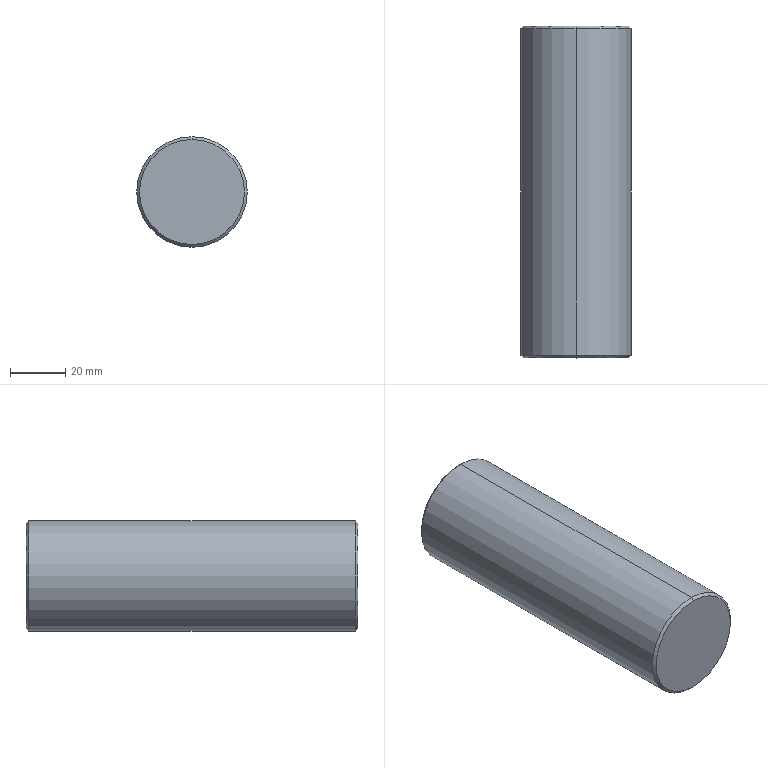Part | SolidWorks | 1 solid | 8 faces | box 40 x 120 x 40 mm | volume 150673 mm3 | cone 4 | cylinder 2 | plane 2 | commonest cylinder face diameters 40 x2
STEP:
#1=CARTESIAN_POINT('',(0.,0.,-19.));
#2=VERTEX_POINT('',#1);
#3=CARTESIAN_POINT('',(0.,0.,19.));
#4=VERTEX_POINT('',#3);
#5=CARTESIAN_POINT('',(0.,0.,0.));
#6=DIRECTION('',(0.,-1.,0.));
#7=DIRECTION('',(0.,0.,-1.));
#8=AXIS2_PLACEMENT_3D('',#5,#6,#7);
#9=CIRCLE('',#8,19.);
#10=EDGE_CURVE('',#2,#4,#9,.T.);
#11=ORIENTED_EDGE('',*,*,#10,.F.);
#12=CARTESIAN_POINT('',(0.,1.,-20.));
#13=VERTEX_POINT('',#12);
#14=CARTESIAN_POINT('',(0.,0.,-19.));
#15=DIRECTION('',(0.,0.7071,-0.7071));
#16=VECTOR('',#15,1000.);
#17=LINE('',#14,#16);
#18=EDGE_CURVE('',#2,#13,#17,.T.);
#19=ORIENTED_EDGE('',*,*,#18,.T.);
#20=CARTESIAN_POINT('',(0.,1.,20.));
#21=VERTEX_POINT('',#20);
#22=CARTESIAN_POINT('',(0.,1.,0.));
#23=DIRECTION('',(0.,-1.,0.));
#24=DIRECTION('',(0.,0.,-1.));
#25=AXIS2_PLACEMENT_3D('',#22,#23,#24);
#26=CIRCLE('',#25,20.);
#27=EDGE_CURVE('',#13,#21,#26,.T.);
#28=ORIENTED_EDGE('',*,*,#27,.T.);
#29=CARTESIAN_POINT('',(0.,0.,19.));
#30=DIRECTION('',(0.,0.7071,0.7071));
#31=VECTOR('',#30,1000.);
#32=LINE('',#29,#31);
#33=EDGE_CURVE('',#4,#21,#32,.T.);
#34=ORIENTED_EDGE('',*,*,#33,.F.);
#35=EDGE_LOOP('',(#11,#19,#28,#34));
#36=FACE_OUTER_BOUND('',#35,.T.);
#37=CARTESIAN_POINT('',(0.,0.,0.));
#38=DIRECTION('',(0.,1.,0.));
#39=DIRECTION('',(0.,0.,1.));
#40=AXIS2_PLACEMENT_3D('',#37,#38,#39);
#41=CONICAL_SURFACE('',#40,19.,0.7854);
#42=ADVANCED_FACE('',(#36),#41,.T.);
#43=CARTESIAN_POINT('',(0.,119.,-20.));
#44=VERTEX_POINT('',#43);
#45=CARTESIAN_POINT('',(0.,119.,20.));
#46=VERTEX_POINT('',#45);
#47=CARTESIAN_POINT('',(0.,119.,0.));
#48=DIRECTION('',(0.,-1.,0.));
#49=DIRECTION('',(0.,0.,-1.));
#50=AXIS2_PLACEMENT_3D('',#47,#48,#49);
#51=CIRCLE('',#50,20.);
#52=EDGE_CURVE('',#44,#46,#51,.T.);
#53=ORIENTED_EDGE('',*,*,#52,.T.);
#54=CARTESIAN_POINT('',(0.,0.,20.));
#55=DIRECTION('',(0.,-1.,0.));
#56=VECTOR('',#55,1000.);
#57=LINE('',#54,#56);
#58=EDGE_CURVE('',#46,#21,#57,.T.);
#59=ORIENTED_EDGE('',*,*,#58,.T.);
#60=ORIENTED_EDGE('',*,*,#27,.F.);
#61=CARTESIAN_POINT('',(0.,0.,-20.));
#62=DIRECTION('',(0.,-1.,0.));
#63=VECTOR('',#62,1000.);
#64=LINE('',#61,#63);
#65=EDGE_CURVE('',#44,#13,#64,.T.);
#66=ORIENTED_EDGE('',*,*,#65,.F.);
#67=EDGE_LOOP('',(#53,#59,#60,#66));
#68=FACE_OUTER_BOUND('',#67,.T.);
#69=CARTESIAN_POINT('',(0.,0.,0.));
#70=DIRECTION('',(0.,-1.,0.));
#71=DIRECTION('',(0.,0.,-1.));
#72=AXIS2_PLACEMENT_3D('',#69,#70,#71);
#73=CYLINDRICAL_SURFACE('',#72,20.);
#74=ADVANCED_FACE('',(#68),#73,.T.);
#75=CARTESIAN_POINT('',(0.,120.,-19.));
#76=VERTEX_POINT('',#75);
#77=CARTESIAN_POINT('',(0.,120.,19.));
#78=VERTEX_POINT('',#77);
#79=CARTESIAN_POINT('',(0.,120.,0.));
#80=DIRECTION('',(0.,-1.,0.));
#81=DIRECTION('',(0.,0.,-1.));
#82=AXIS2_PLACEMENT_3D('',#79,#80,#81);
#83=CIRCLE('',#82,19.);
#84=EDGE_CURVE('',#76,#78,#83,.T.);
#85=ORIENTED_EDGE('',*,*,#84,.T.);
#86=CARTESIAN_POINT('',(0.,119.,20.));
#87=DIRECTION('',(0.,-0.7071,0.7071));
#88=VECTOR('',#87,1000.);
#89=LINE('',#86,#88);
#90=EDGE_CURVE('',#78,#46,#89,.T.);
#91=ORIENTED_EDGE('',*,*,#90,.T.);
#92=ORIENTED_EDGE('',*,*,#52,.F.);
#93=CARTESIAN_POINT('',(0.,119.,-20.));
#94=DIRECTION('',(0.,-0.7071,-0.7071));
#95=VECTOR('',#94,1000.);
#96=LINE('',#93,#95);
#97=EDGE_CURVE('',#76,#44,#96,.T.);
#98=ORIENTED_EDGE('',*,*,#97,.F.);
#99=EDGE_LOOP('',(#85,#91,#92,#98));
#100=FACE_OUTER_BOUND('',#99,.T.);
#101=CARTESIAN_POINT('',(0.,119.,0.));
#102=DIRECTION('',(0.,-1.,0.));
#103=DIRECTION('',(0.,0.,-1.));
#104=AXIS2_PLACEMENT_3D('',#101,#102,#103);
#105=CONICAL_SURFACE('',#104,20.,0.7854);
#106=ADVANCED_FACE('',(#100),#105,.T.);
#107=ORIENTED_EDGE('',*,*,#84,.F.);
#108=CARTESIAN_POINT('',(0.,120.,0.));
#109=DIRECTION('',(0.,-1.,0.));
#110=DIRECTION('',(0.,0.,-1.));
#111=AXIS2_PLACEMENT_3D('',#108,#109,#110);
#112=CIRCLE('',#111,19.);
#113=EDGE_CURVE('',#78,#76,#112,.T.);
#114=ORIENTED_EDGE('',*,*,#113,.F.);
#115=EDGE_LOOP('',(#107,#114));
#116=FACE_OUTER_BOUND('',#115,.T.);
#117=CARTESIAN_POINT('',(0.,120.,0.));
#118=DIRECTION('',(0.,1.,0.));
#119=DIRECTION('',(0.,0.,1.));
#120=AXIS2_PLACEMENT_3D('',#117,#118,#119);
#121=PLANE('',#120);
#122=ADVANCED_FACE('',(#116),#121,.T.);
#123=ORIENTED_EDGE('',*,*,#90,.F.);
#124=ORIENTED_EDGE('',*,*,#113,.T.);
#125=ORIENTED_EDGE('',*,*,#97,.T.);
#126=CARTESIAN_POINT('',(0.,119.,0.));
#127=DIRECTION('',(0.,-1.,0.));
#128=DIRECTION('',(0.,0.,-1.));
#129=AXIS2_PLACEMENT_3D('',#126,#127,#128);
#130=CIRCLE('',#129,20.);
#131=EDGE_CURVE('',#46,#44,#130,.T.);
#132=ORIENTED_EDGE('',*,*,#131,.F.);
#133=EDGE_LOOP('',(#123,#124,#125,#132));
#134=FACE_OUTER_BOUND('',#133,.T.);
#135=CARTESIAN_POINT('',(0.,119.,0.));
#136=DIRECTION('',(0.,-1.,0.));
#137=DIRECTION('',(0.,0.,-1.));
#138=AXIS2_PLACEMENT_3D('',#135,#136,#137);
#139=CONICAL_SURFACE('',#138,20.,0.7854);
#140=ADVANCED_FACE('',(#134),#139,.T.);
#141=ORIENTED_EDGE('',*,*,#58,.F.);
#142=ORIENTED_EDGE('',*,*,#131,.T.);
#143=ORIENTED_EDGE('',*,*,#65,.T.);
#144=CARTESIAN_POINT('',(0.,1.,0.));
#145=DIRECTION('',(0.,-1.,0.));
#146=DIRECTION('',(0.,0.,-1.));
#147=AXIS2_PLACEMENT_3D('',#144,#145,#146);
#148=CIRCLE('',#147,20.);
#149=EDGE_CURVE('',#21,#13,#148,.T.);
#150=ORIENTED_EDGE('',*,*,#149,.F.);
#151=EDGE_LOOP('',(#141,#142,#143,#150));
#152=FACE_OUTER_BOUND('',#151,.T.);
#153=CARTESIAN_POINT('',(0.,0.,0.));
#154=DIRECTION('',(0.,-1.,0.));
#155=DIRECTION('',(0.,0.,-1.));
#156=AXIS2_PLACEMENT_3D('',#153,#154,#155);
#157=CYLINDRICAL_SURFACE('',#156,20.);
#158=ADVANCED_FACE('',(#152),#157,.T.);
#159=ORIENTED_EDGE('',*,*,#18,.F.);
#160=CARTESIAN_POINT('',(0.,0.,0.));
#161=DIRECTION('',(0.,-1.,0.));
#162=DIRECTION('',(0.,0.,-1.));
#163=AXIS2_PLACEMENT_3D('',#160,#161,#162);
#164=CIRCLE('',#163,19.);
#165=EDGE_CURVE('',#4,#2,#164,.T.);
#166=ORIENTED_EDGE('',*,*,#165,.F.);
#167=ORIENTED_EDGE('',*,*,#33,.T.);
#168=ORIENTED_EDGE('',*,*,#149,.T.);
#169=EDGE_LOOP('',(#159,#166,#167,#168));
#170=FACE_OUTER_BOUND('',#169,.T.);
#171=CARTESIAN_POINT('',(0.,0.,0.));
#172=DIRECTION('',(0.,1.,0.));
#173=DIRECTION('',(0.,0.,1.));
#174=AXIS2_PLACEMENT_3D('',#171,#172,#173);
#175=CONICAL_SURFACE('',#174,19.,0.7854);
#176=ADVANCED_FACE('',(#170),#175,.T.);
#177=ORIENTED_EDGE('',*,*,#165,.T.);
#178=ORIENTED_EDGE('',*,*,#10,.T.);
#179=EDGE_LOOP('',(#177,#178));
#180=FACE_OUTER_BOUND('',#179,.T.);
#181=CARTESIAN_POINT('',(0.,0.,0.));
#182=DIRECTION('',(0.,-1.,0.));
#183=DIRECTION('',(0.,0.,-1.));
#184=AXIS2_PLACEMENT_3D('',#181,#182,#183);
#185=PLANE('',#184);
#186=ADVANCED_FACE('',(#180),#185,.T.);
#187=CLOSED_SHELL('',(#42,#74,#106,#122,#140,#158,#176,#186));
#188=MANIFOLD_SOLID_BREP('',#187);
#189=CARTESIAN_POINT('',(0.,0.,0.));
#190=DIRECTION('',(0.,0.,1.));
#191=DIRECTION('',(1.,0.,0.));
#192=AXIS2_PLACEMENT_3D('',#189,#190,#191);
#193=(LENGTH_UNIT()NAMED_UNIT(*)SI_UNIT(.MILLI.,.METRE.));
#194=UNCERTAINTY_MEASURE_WITH_UNIT(LENGTH_MEASURE(0.00001),#193,'','');
#195=(NAMED_UNIT(*)PLANE_ANGLE_UNIT()SI_UNIT($,.RADIAN.));
#196=(NAMED_UNIT(*)SI_UNIT($,.STERADIAN.)SOLID_ANGLE_UNIT());
#197=(GEOMETRIC_REPRESENTATION_CONTEXT(3)GLOBAL_UNCERTAINTY_ASSIGNED_CONTEXT((#194))GLOBAL_UNIT_ASSIGNED_CONTEXT((#193,#195,#196))REPRESENTATION_CONTEXT('',''));
#198=ADVANCED_BREP_SHAPE_REPRESENTATION('',(#188,#192),#197);